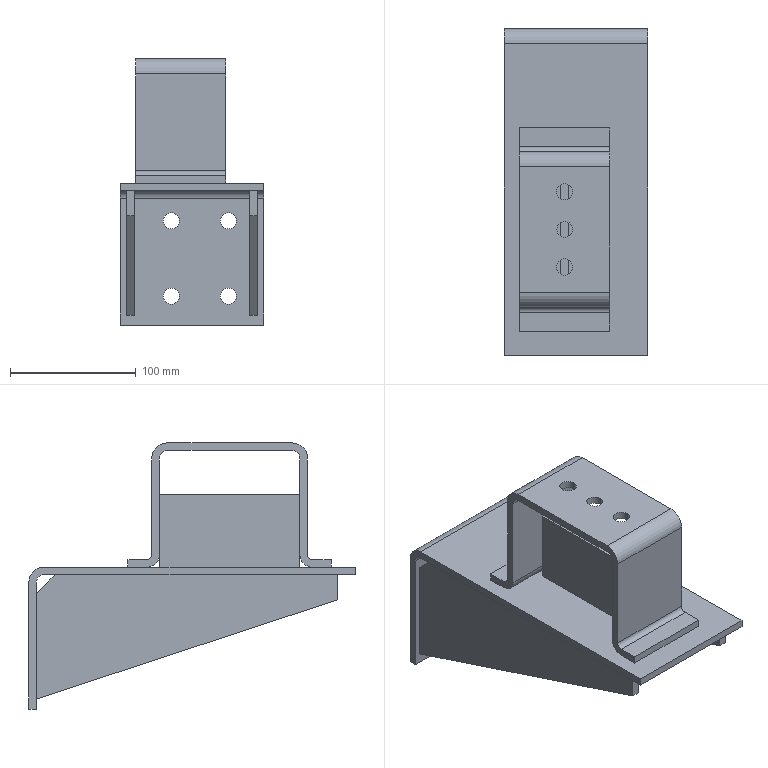Part | NX | features BREP 5 | 5 solids | 66 faces | box 114 x 260 x 212 mm | volume 596260 mm3 | plane 42 | cylinder 24 | commonest cylinder face diameters 13 x12 12 x3 24 x3 8 x2 12.5 x2 20 x2